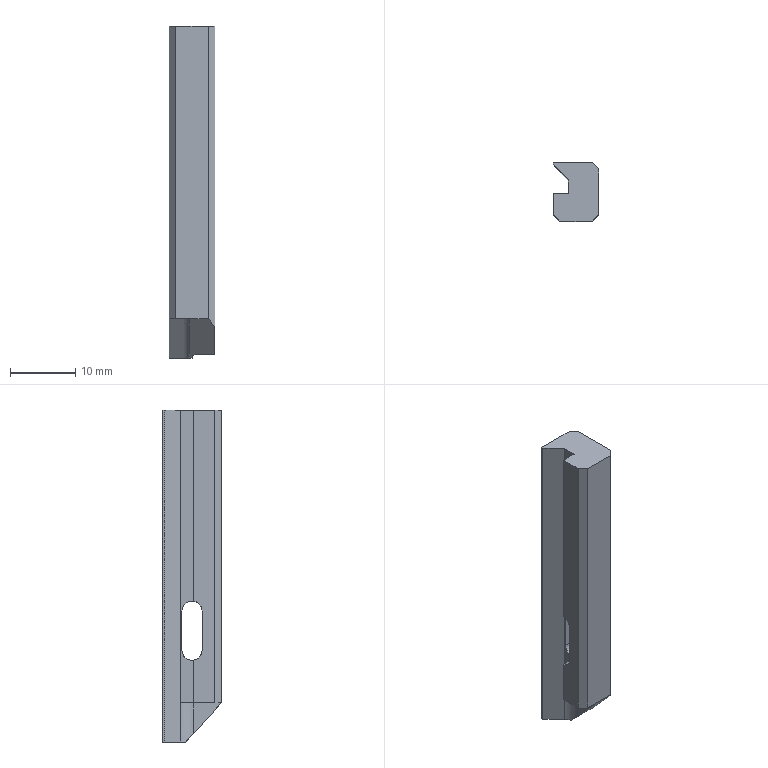Part | STEP file | 03-14 trimming upper-right blade | 1 solid | 30 faces | box 7 x 9 x 51 mm | volume 2452 mm3 | plane 22 | cylinder 8 | commonest cylinder face diameters 0.7 x4 3.1 x2 1 x1 6 x1
STEP:
#1=CARTESIAN_POINT('',(0.2245,4.1,1.));
#2=VERTEX_POINT('',#1);
#3=CARTESIAN_POINT('',(-0.4755,4.1,1.));
#4=VERTEX_POINT('',#3);
#5=CARTESIAN_POINT('',(-0.1255,4.1,1.));
#6=DIRECTION('',(0.,0.,-1.));
#7=DIRECTION('',(-1.,0.,0.));
#8=AXIS2_PLACEMENT_3D('',#5,#6,#7);
#9=CIRCLE('',#8,0.35);
#10=EDGE_CURVE('',#2,#4,#9,.T.);
#11=ORIENTED_EDGE('',*,*,#10,.F.);
#12=CARTESIAN_POINT('',(0.2245,4.1,0.));
#13=VERTEX_POINT('',#12);
#14=CARTESIAN_POINT('',(0.2245,4.1,1.));
#15=DIRECTION('',(0.,0.,-1.));
#16=VECTOR('',#15,1000.);
#17=LINE('',#14,#16);
#18=EDGE_CURVE('',#2,#13,#17,.T.);
#19=ORIENTED_EDGE('',*,*,#18,.T.);
#20=CARTESIAN_POINT('',(-0.4755,4.1,0.));
#21=VERTEX_POINT('',#20);
#22=CARTESIAN_POINT('',(-0.1255,4.1,0.));
#23=DIRECTION('',(0.,0.,-1.));
#24=DIRECTION('',(-1.,0.,0.));
#25=AXIS2_PLACEMENT_3D('',#22,#23,#24);
#26=CIRCLE('',#25,0.35);
#27=EDGE_CURVE('',#13,#21,#26,.T.);
#28=ORIENTED_EDGE('',*,*,#27,.T.);
#29=CARTESIAN_POINT('',(-0.4755,4.1,1.));
#30=DIRECTION('',(0.,0.,-1.));
#31=VECTOR('',#30,1000.);
#32=LINE('',#29,#31);
#33=EDGE_CURVE('',#4,#21,#32,.T.);
#34=ORIENTED_EDGE('',*,*,#33,.F.);
#35=EDGE_LOOP('',(#11,#19,#28,#34));
#36=FACE_OUTER_BOUND('',#35,.T.);
#37=CARTESIAN_POINT('',(-0.1255,4.1,1.));
#38=DIRECTION('',(0.,0.,-1.));
#39=DIRECTION('',(-1.,0.,0.));
#40=AXIS2_PLACEMENT_3D('',#37,#38,#39);
#41=CYLINDRICAL_SURFACE('',#40,0.35);
#42=ADVANCED_FACE('',(#36),#41,.F.);
#43=CARTESIAN_POINT('',(1.524,4.1,1.));
#44=VERTEX_POINT('',#43);
#45=CARTESIAN_POINT('',(0.8245,4.1,1.));
#46=VERTEX_POINT('',#45);
#47=CARTESIAN_POINT('',(1.174,4.1,1.));
#48=DIRECTION('',(0.,0.,-1.));
#49=DIRECTION('',(-1.,0.,0.));
#50=AXIS2_PLACEMENT_3D('',#47,#48,#49);
#51=CIRCLE('',#50,0.35);
#52=EDGE_CURVE('',#44,#46,#51,.T.);
#53=ORIENTED_EDGE('',*,*,#52,.F.);
#54=CARTESIAN_POINT('',(1.524,4.1,0.));
#55=VERTEX_POINT('',#54);
#56=CARTESIAN_POINT('',(1.524,4.1,1.));
#57=DIRECTION('',(0.,0.,-1.));
#58=VECTOR('',#57,1000.);
#59=LINE('',#56,#58);
#60=EDGE_CURVE('',#44,#55,#59,.T.);
#61=ORIENTED_EDGE('',*,*,#60,.T.);
#62=CARTESIAN_POINT('',(0.8245,4.1,0.));
#63=VERTEX_POINT('',#62);
#64=CARTESIAN_POINT('',(1.174,4.1,0.));
#65=DIRECTION('',(0.,0.,-1.));
#66=DIRECTION('',(-1.,0.,0.));
#67=AXIS2_PLACEMENT_3D('',#64,#65,#66);
#68=CIRCLE('',#67,0.35);
#69=EDGE_CURVE('',#55,#63,#68,.T.);
#70=ORIENTED_EDGE('',*,*,#69,.T.);
#71=CARTESIAN_POINT('',(0.8245,4.1,1.));
#72=DIRECTION('',(0.,0.,-1.));
#73=VECTOR('',#72,1000.);
#74=LINE('',#71,#73);
#75=EDGE_CURVE('',#46,#63,#74,.T.);
#76=ORIENTED_EDGE('',*,*,#75,.F.);
#77=EDGE_LOOP('',(#53,#61,#70,#76));
#78=FACE_OUTER_BOUND('',#77,.T.);
#79=CARTESIAN_POINT('',(1.174,4.1,1.));
#80=DIRECTION('',(0.,0.,-1.));
#81=DIRECTION('',(-1.,0.,0.));
#82=AXIS2_PLACEMENT_3D('',#79,#80,#81);
#83=CYLINDRICAL_SURFACE('',#82,0.35);
#84=ADVANCED_FACE('',(#78),#83,.F.);
#85=CARTESIAN_POINT('',(1.311,-0.2729,51.));
#86=VERTEX_POINT('',#85);
#87=CARTESIAN_POINT('',(1.311,-0.2729,21.626));
#88=VERTEX_POINT('',#87);
#89=CARTESIAN_POINT('',(1.311,-0.2729,51.));
#90=DIRECTION('',(0.,0.,-1.));
#91=VECTOR('',#90,1000.);
#92=LINE('',#89,#91);
#93=EDGE_CURVE('',#86,#88,#92,.T.);
#94=ORIENTED_EDGE('',*,*,#93,.T.);
#95=CARTESIAN_POINT('',(-1.,-0.2729,21.626));
#96=VERTEX_POINT('',#95);
#97=CARTESIAN_POINT('',(-16.,-0.2729,21.626));
#98=DIRECTION('',(-1.,0.,0.));
#99=VECTOR('',#98,1000.);
#100=LINE('',#97,#99);
#101=EDGE_CURVE('',#88,#96,#100,.T.);
#102=ORIENTED_EDGE('',*,*,#101,.T.);
#103=CARTESIAN_POINT('',(-1.,-0.2729,51.));
#104=VERTEX_POINT('',#103);
#105=CARTESIAN_POINT('',(-1.,-0.2729,51.));
#106=DIRECTION('',(0.,0.,1.));
#107=VECTOR('',#106,1000.);
#108=LINE('',#105,#107);
#109=EDGE_CURVE('',#96,#104,#108,.T.);
#110=ORIENTED_EDGE('',*,*,#109,.T.);
#111=CARTESIAN_POINT('',(1.311,-0.2729,51.));
#112=DIRECTION('',(-1.,0.,0.));
#113=VECTOR('',#112,1000.);
#114=LINE('',#111,#113);
#115=EDGE_CURVE('',#86,#104,#114,.T.);
#116=ORIENTED_EDGE('',*,*,#115,.F.);
#117=EDGE_LOOP('',(#94,#102,#110,#116));
#118=FACE_OUTER_BOUND('',#117,.T.);
#119=CARTESIAN_POINT('',(1.311,-0.2729,51.));
#120=DIRECTION('',(0.,-1.,0.));
#121=DIRECTION('',(1.,0.,0.));
#122=AXIS2_PLACEMENT_3D('',#119,#120,#121);
#123=PLANE('',#122);
#124=ADVANCED_FACE('',(#118),#123,.F.);
#125=CARTESIAN_POINT('',(5.,4.5,51.));
#126=VERTEX_POINT('',#125);
#127=CARTESIAN_POINT('',(5.,4.5,0.5));
#128=VERTEX_POINT('',#127);
#129=CARTESIAN_POINT('',(5.,4.5,51.));
#130=DIRECTION('',(0.,0.,-1.));
#131=VECTOR('',#130,1000.);
#132=LINE('',#129,#131);
#133=EDGE_CURVE('',#126,#128,#132,.T.);
#134=ORIENTED_EDGE('',*,*,#133,.T.);
#135=CARTESIAN_POINT('',(3.,4.5,0.5));
#136=VERTEX_POINT('',#135);
#137=CARTESIAN_POINT('',(6.,4.5,0.5));
#138=DIRECTION('',(1.,0.,0.));
#139=VECTOR('',#138,1000.);
#140=LINE('',#137,#139);
#141=EDGE_CURVE('',#136,#128,#140,.T.);
#142=ORIENTED_EDGE('',*,*,#141,.F.);
#143=CARTESIAN_POINT('',(2.5,4.5,0.));
#144=VERTEX_POINT('',#143);
#145=CARTESIAN_POINT('',(3.,4.5,0.));
#146=DIRECTION('',(0.,-1.,0.));
#147=DIRECTION('',(0.,0.,-1.));
#148=AXIS2_PLACEMENT_3D('',#145,#146,#147);
#149=CIRCLE('',#148,0.5);
#150=EDGE_CURVE('',#136,#144,#149,.T.);
#151=ORIENTED_EDGE('',*,*,#150,.T.);
#152=CARTESIAN_POINT('',(-1.,4.5,0.));
#153=VERTEX_POINT('',#152);
#154=CARTESIAN_POINT('',(-6.,4.5,0.));
#155=DIRECTION('',(-1.,0.,0.));
#156=VECTOR('',#155,1000.);
#157=LINE('',#154,#156);
#158=EDGE_CURVE('',#144,#153,#157,.T.);
#159=ORIENTED_EDGE('',*,*,#158,.T.);
#160=CARTESIAN_POINT('',(-1.,4.5,51.));
#161=VERTEX_POINT('',#160);
#162=CARTESIAN_POINT('',(-1.,4.5,51.));
#163=DIRECTION('',(0.,0.,-1.));
#164=VECTOR('',#163,1000.);
#165=LINE('',#162,#164);
#166=EDGE_CURVE('',#161,#153,#165,.T.);
#167=ORIENTED_EDGE('',*,*,#166,.F.);
#168=CARTESIAN_POINT('',(-6.,4.5,51.));
#169=DIRECTION('',(-1.,0.,0.));
#170=VECTOR('',#169,1000.);
#171=LINE('',#168,#170);
#172=EDGE_CURVE('',#126,#161,#171,.T.);
#173=ORIENTED_EDGE('',*,*,#172,.F.);
#174=EDGE_LOOP('',(#134,#142,#151,#159,#167,#173));
#175=FACE_OUTER_BOUND('',#174,.T.);
#176=CARTESIAN_POINT('',(-6.,4.5,51.));
#177=DIRECTION('',(0.,-1.,0.));
#178=DIRECTION('',(0.,0.,-1.));
#179=AXIS2_PLACEMENT_3D('',#176,#177,#178);
#180=PLANE('',#179);
#181=ADVANCED_FACE('',(#175),#180,.F.);
#182=CARTESIAN_POINT('',(-0.1255,4.1,0.));
#183=DIRECTION('',(0.,0.,-1.));
#184=DIRECTION('',(-1.,0.,0.));
#185=AXIS2_PLACEMENT_3D('',#182,#183,#184);
#186=CIRCLE('',#185,0.35);
#187=EDGE_CURVE('',#21,#13,#186,.T.);
#188=ORIENTED_EDGE('',*,*,#187,.F.);
#189=ORIENTED_EDGE('',*,*,#27,.F.);
#190=EDGE_LOOP('',(#188,#189));
#191=FACE_BOUND('',#190,.T.);
#192=CARTESIAN_POINT('',(1.174,4.1,0.));
#193=DIRECTION('',(0.,0.,-1.));
#194=DIRECTION('',(-1.,0.,0.));
#195=AXIS2_PLACEMENT_3D('',#192,#193,#194);
#196=CIRCLE('',#195,0.35);
#197=EDGE_CURVE('',#63,#55,#196,.T.);
#198=ORIENTED_EDGE('',*,*,#197,.F.);
#199=ORIENTED_EDGE('',*,*,#69,.F.);
#200=EDGE_LOOP('',(#198,#199));
#201=FACE_BOUND('',#200,.T.);
#202=ORIENTED_EDGE('',*,*,#158,.F.);
#203=CARTESIAN_POINT('',(2.5,0.9407,0.));
#204=VERTEX_POINT('',#203);
#205=CARTESIAN_POINT('',(2.5,-0.5,0.));
#206=DIRECTION('',(0.,1.,0.));
#207=VECTOR('',#206,1000.);
#208=LINE('',#205,#207);
#209=EDGE_CURVE('',#204,#144,#208,.T.);
#210=ORIENTED_EDGE('',*,*,#209,.F.);
#211=CARTESIAN_POINT('',(1.899,0.9407,0.));
#212=VERTEX_POINT('',#211);
#213=CARTESIAN_POINT('',(6.663,0.9407,0.));
#214=DIRECTION('',(1.,0.,0.));
#215=VECTOR('',#214,1000.);
#216=LINE('',#213,#215);
#217=EDGE_CURVE('',#212,#204,#216,.T.);
#218=ORIENTED_EDGE('',*,*,#217,.F.);
#219=CARTESIAN_POINT('',(1.311,1.813,0.));
#220=VERTEX_POINT('',#219);
#221=CARTESIAN_POINT('',(-0.8447,-0.2729,0.));
#222=DIRECTION('',(0.,0.,1.));
#223=DIRECTION('',(1.,0.,0.));
#224=AXIS2_PLACEMENT_3D('',#221,#222,#223);
#225=CIRCLE('',#224,3.);
#226=EDGE_CURVE('',#212,#220,#225,.T.);
#227=ORIENTED_EDGE('',*,*,#226,.T.);
#228=CARTESIAN_POINT('',(-1.,4.202,0.));
#229=VERTEX_POINT('',#228);
#230=CARTESIAN_POINT('',(6.733,-3.791,0.));
#231=DIRECTION('',(-0.6953,0.7187,0.));
#232=VECTOR('',#231,1000.);
#233=LINE('',#230,#232);
#234=EDGE_CURVE('',#220,#229,#233,.T.);
#235=ORIENTED_EDGE('',*,*,#234,.T.);
#236=CARTESIAN_POINT('',(-1.,-4.5,0.));
#237=DIRECTION('',(0.,-1.,0.));
#238=VECTOR('',#237,1000.);
#239=LINE('',#236,#238);
#240=EDGE_CURVE('',#153,#229,#239,.T.);
#241=ORIENTED_EDGE('',*,*,#240,.F.);
#242=EDGE_LOOP('',(#202,#210,#218,#227,#235,#241));
#243=FACE_OUTER_BOUND('',#242,.T.);
#244=CARTESIAN_POINT('',(6.,-4.5,0.));
#245=DIRECTION('',(0.,0.,1.));
#246=DIRECTION('',(1.,0.,0.));
#247=AXIS2_PLACEMENT_3D('',#244,#245,#246);
#248=PLANE('',#247);
#249=ADVANCED_FACE('',(#191,#201,#243),#248,.F.);
#250=ORIENTED_EDGE('',*,*,#234,.F.);
#251=CARTESIAN_POINT('',(1.311,1.813,6.));
#252=VERTEX_POINT('',#251);
#253=CARTESIAN_POINT('',(1.311,1.813,6.));
#254=DIRECTION('',(0.,0.,1.));
#255=VECTOR('',#254,1000.);
#256=LINE('',#253,#255);
#257=EDGE_CURVE('',#220,#252,#256,.T.);
#258=ORIENTED_EDGE('',*,*,#257,.T.);
#259=CARTESIAN_POINT('',(1.311,1.813,51.));
#260=VERTEX_POINT('',#259);
#261=CARTESIAN_POINT('',(1.311,1.813,51.));
#262=DIRECTION('',(0.,0.,-1.));
#263=VECTOR('',#262,1000.);
#264=LINE('',#261,#263);
#265=EDGE_CURVE('',#260,#252,#264,.T.);
#266=ORIENTED_EDGE('',*,*,#265,.F.);
#267=CARTESIAN_POINT('',(-1.,4.202,51.));
#268=VERTEX_POINT('',#267);
#269=CARTESIAN_POINT('',(-1.,4.202,51.));
#270=DIRECTION('',(0.6953,-0.7187,0.));
#271=VECTOR('',#270,1000.);
#272=LINE('',#269,#271);
#273=EDGE_CURVE('',#268,#260,#272,.T.);
#274=ORIENTED_EDGE('',*,*,#273,.F.);
#275=CARTESIAN_POINT('',(-1.,4.202,6.));
#276=DIRECTION('',(0.,0.,1.));
#277=VECTOR('',#276,1000.);
#278=LINE('',#275,#277);
#279=EDGE_CURVE('',#229,#268,#278,.T.);
#280=ORIENTED_EDGE('',*,*,#279,.F.);
#281=EDGE_LOOP('',(#250,#258,#266,#274,#280));
#282=FACE_OUTER_BOUND('',#281,.T.);
#283=CARTESIAN_POINT('',(-2.682,5.941,6.));
#284=DIRECTION('',(0.7187,0.6953,0.));
#285=DIRECTION('',(-0.6953,0.7187,0.));
#286=AXIS2_PLACEMENT_3D('',#283,#284,#285);
#287=PLANE('',#286);
#288=ADVANCED_FACE('',(#282),#287,.F.);
#289=CARTESIAN_POINT('',(6.,0.4873,0.5));
#290=VERTEX_POINT('',#289);
#291=CARTESIAN_POINT('',(3.,0.4873,0.5));
#292=VERTEX_POINT('',#291);
#293=CARTESIAN_POINT('',(-6.,0.4873,0.5));
#294=DIRECTION('',(-1.,0.,0.));
#295=VECTOR('',#294,1000.);
#296=LINE('',#293,#295);
#297=EDGE_CURVE('',#290,#292,#296,.T.);
#298=ORIENTED_EDGE('',*,*,#297,.F.);
#299=CARTESIAN_POINT('',(6.,-3.5,4.897));
#300=VERTEX_POINT('',#299);
#301=CARTESIAN_POINT('',(6.,0.9407,0.));
#302=DIRECTION('',(0.,0.6717,-0.7408));
#303=VECTOR('',#302,1000.);
#304=LINE('',#301,#303);
#305=EDGE_CURVE('',#300,#290,#304,.T.);
#306=ORIENTED_EDGE('',*,*,#305,.F.);
#307=CARTESIAN_POINT('',(5.,-4.5,6.));
#308=VERTEX_POINT('',#307);
#309=CARTESIAN_POINT('',(5.329,-4.171,5.637));
#310=DIRECTION('',(-0.5576,-0.5576,0.6149));
#311=VECTOR('',#310,1000.);
#312=LINE('',#309,#311);
#313=EDGE_CURVE('',#300,#308,#312,.T.);
#314=ORIENTED_EDGE('',*,*,#313,.T.);
#315=CARTESIAN_POINT('',(2.155,-4.5,6.));
#316=VERTEX_POINT('',#315);
#317=CARTESIAN_POINT('',(-6.,-4.5,6.));
#318=DIRECTION('',(1.,0.,0.));
#319=VECTOR('',#318,1000.);
#320=LINE('',#317,#319);
#321=EDGE_CURVE('',#316,#308,#320,.T.);
#322=ORIENTED_EDGE('',*,*,#321,.F.);
#323=CARTESIAN_POINT('',(2.155,-0.2729,1.338));
#324=VERTEX_POINT('',#323);
#325=CARTESIAN_POINT('',(2.155,0.9407,0.));
#326=DIRECTION('',(0.,0.6717,-0.7408));
#327=VECTOR('',#326,1000.);
#328=LINE('',#325,#327);
#329=EDGE_CURVE('',#316,#324,#328,.T.);
#330=ORIENTED_EDGE('',*,*,#329,.T.);
#331=CARTESIAN_POINT('',(2.155,-0.2729,1.338));
#332=CARTESIAN_POINT('',(2.155,0.1466,0.8758));
#333=CARTESIAN_POINT('',(2.069,0.5571,0.4231));
#334=CARTESIAN_POINT('',(1.899,0.9407,0.));
#335=(BOUNDED_CURVE()B_SPLINE_CURVE(3,(#331,#332,#333,#334),.UNSPECIFIED.,.F.,.F.)B_SPLINE_CURVE_WITH_KNOTS((4,4),(4.712,5.129),.UNSPECIFIED.)CURVE()GEOMETRIC_REPRESENTATION_ITEM()RATIONAL_B_SPLINE_CURVE((1.,0.9856,0.9856,1.))REPRESENTATION_ITEM(''));
#336=EDGE_CURVE('',#324,#212,#335,.T.);
#337=ORIENTED_EDGE('',*,*,#336,.T.);
#338=ORIENTED_EDGE('',*,*,#217,.T.);
#339=CARTESIAN_POINT('',(2.5,0.9407,0.));
#340=CARTESIAN_POINT('',(2.5,0.6751,0.2929));
#341=CARTESIAN_POINT('',(2.707,0.4873,0.5));
#342=CARTESIAN_POINT('',(3.,0.4873,0.5));
#343=(BOUNDED_CURVE()B_SPLINE_CURVE(3,(#339,#340,#341,#342),.UNSPECIFIED.,.F.,.F.)B_SPLINE_CURVE_WITH_KNOTS((4,4),(4.712,6.283),.UNSPECIFIED.)CURVE()GEOMETRIC_REPRESENTATION_ITEM()RATIONAL_B_SPLINE_CURVE((1.,0.8047,0.8047,1.))REPRESENTATION_ITEM(''));
#344=EDGE_CURVE('',#204,#292,#343,.T.);
#345=ORIENTED_EDGE('',*,*,#344,.T.);
#346=EDGE_LOOP('',(#298,#306,#314,#322,#330,#337,#338,#345));
#347=FACE_OUTER_BOUND('',#346,.T.);
#348=CARTESIAN_POINT('',(-6.,0.9407,0.));
#349=DIRECTION('',(0.,-0.7408,-0.6717));
#350=DIRECTION('',(0.,0.6717,-0.7408));
#351=AXIS2_PLACEMENT_3D('',#348,#349,#350);
#352=PLANE('',#351);
#353=ADVANCED_FACE('',(#347),#352,.T.);
#354=CARTESIAN_POINT('',(6.,-1.55,20.1));
#355=VERTEX_POINT('',#354);
#356=CARTESIAN_POINT('',(6.,-1.55,14.1));
#357=VERTEX_POINT('',#356);
#358=CARTESIAN_POINT('',(6.,-1.55,20.1));
#359=DIRECTION('',(0.,0.,-1.));
#360=VECTOR('',#359,1000.);
#361=LINE('',#358,#360);
#362=EDGE_CURVE('',#355,#357,#361,.T.);
#363=ORIENTED_EDGE('',*,*,#362,.F.);
#364=CARTESIAN_POINT('',(6.,1.55,20.1));
#365=VERTEX_POINT('',#364);
#366=CARTESIAN_POINT('',(6.,0.,20.1));
#367=DIRECTION('',(1.,0.,0.));
#368=DIRECTION('',(0.,1.,0.));
#369=AXIS2_PLACEMENT_3D('',#366,#367,#368);
#370=CIRCLE('',#369,1.55);
#371=EDGE_CURVE('',#365,#355,#370,.T.);
#372=ORIENTED_EDGE('',*,*,#371,.F.);
#373=CARTESIAN_POINT('',(6.,1.55,14.1));
#374=VERTEX_POINT('',#373);
#375=CARTESIAN_POINT('',(6.,1.55,20.1));
#376=DIRECTION('',(0.,0.,1.));
#377=VECTOR('',#376,1000.);
#378=LINE('',#375,#377);
#379=EDGE_CURVE('',#374,#365,#378,.T.);
#380=ORIENTED_EDGE('',*,*,#379,.F.);
#381=CARTESIAN_POINT('',(6.,0.,14.1));
#382=DIRECTION('',(1.,0.,0.));
#383=DIRECTION('',(0.,1.,0.));
#384=AXIS2_PLACEMENT_3D('',#381,#382,#383);
#385=CIRCLE('',#384,1.55);
#386=EDGE_CURVE('',#357,#374,#385,.T.);
#387=ORIENTED_EDGE('',*,*,#386,.F.);
#388=EDGE_LOOP('',(#363,#372,#380,#387));
#389=FACE_BOUND('',#388,.T.);
#390=ORIENTED_EDGE('',*,*,#305,.T.);
#391=CARTESIAN_POINT('',(6.,3.5,0.5));
#392=VERTEX_POINT('',#391);
#393=CARTESIAN_POINT('',(6.,-0.5,0.5));
#394=DIRECTION('',(0.,1.,0.));
#395=VECTOR('',#394,1000.);
#396=LINE('',#393,#395);
#397=EDGE_CURVE('',#290,#392,#396,.T.);
#398=ORIENTED_EDGE('',*,*,#397,.T.);
#399=CARTESIAN_POINT('',(6.,3.5,51.));
#400=VERTEX_POINT('',#399);
#401=CARTESIAN_POINT('',(6.,3.5,51.));
#402=DIRECTION('',(0.,0.,1.));
#403=VECTOR('',#402,1000.);
#404=LINE('',#401,#403);
#405=EDGE_CURVE('',#392,#400,#404,.T.);
#406=ORIENTED_EDGE('',*,*,#405,.T.);
#407=CARTESIAN_POINT('',(6.,-3.5,51.));
#408=VERTEX_POINT('',#407);
#409=CARTESIAN_POINT('',(6.,4.5,51.));
#410=DIRECTION('',(0.,1.,0.));
#411=VECTOR('',#410,1000.);
#412=LINE('',#409,#411);
#413=EDGE_CURVE('',#408,#400,#412,.T.);
#414=ORIENTED_EDGE('',*,*,#413,.F.);
#415=CARTESIAN_POINT('',(6.,-3.5,51.));
#416=DIRECTION('',(0.,0.,-1.));
#417=VECTOR('',#416,1000.);
#418=LINE('',#415,#417);
#419=EDGE_CURVE('',#408,#300,#418,.T.);
#420=ORIENTED_EDGE('',*,*,#419,.T.);
#421=EDGE_LOOP('',(#390,#398,#406,#414,#420));
#422=FACE_OUTER_BOUND('',#421,.T.);
#423=CARTESIAN_POINT('',(6.,4.5,51.));
#424=DIRECTION('',(-1.,0.,0.));
#425=DIRECTION('',(0.,-1.,0.));
#426=AXIS2_PLACEMENT_3D('',#423,#424,#425);
#427=PLANE('',#426);
#428=ADVANCED_FACE('',(#389,#422),#427,.F.);
#429=CARTESIAN_POINT('',(0.,-4.5,51.));
#430=VERTEX_POINT('',#429);
#431=CARTESIAN_POINT('',(5.,-4.5,51.));
#432=VERTEX_POINT('',#431);
#433=CARTESIAN_POINT('',(-6.,-4.5,51.));
#434=DIRECTION('',(1.,0.,0.));
#435=VECTOR('',#434,1000.);
#436=LINE('',#433,#435);
#437=EDGE_CURVE('',#430,#432,#436,.T.);
#438=ORIENTED_EDGE('',*,*,#437,.F.);
#439=CARTESIAN_POINT('',(0.,-4.5,6.));
#440=VERTEX_POINT('',#439);
#441=CARTESIAN_POINT('',(0.,-4.5,51.));
#442=DIRECTION('',(0.,0.,-1.));
#443=VECTOR('',#442,1000.);
#444=LINE('',#441,#443);
#445=EDGE_CURVE('',#430,#440,#444,.T.);
#446=ORIENTED_EDGE('',*,*,#445,.T.);
#447=CARTESIAN_POINT('',(-6.,-4.5,6.));
#448=DIRECTION('',(1.,0.,0.));
#449=VECTOR('',#448,1000.);
#450=LINE('',#447,#449);
#451=EDGE_CURVE('',#440,#316,#450,.T.);
#452=ORIENTED_EDGE('',*,*,#451,.T.);
#453=ORIENTED_EDGE('',*,*,#321,.T.);
#454=CARTESIAN_POINT('',(5.,-4.5,51.));
#455=DIRECTION('',(0.,0.,1.));
#456=VECTOR('',#455,1000.);
#457=LINE('',#454,#456);
#458=EDGE_CURVE('',#308,#432,#457,.T.);
#459=ORIENTED_EDGE('',*,*,#458,.T.);
#460=EDGE_LOOP('',(#438,#446,#452,#453,#459));
#461=FACE_OUTER_BOUND('',#460,.T.);
#462=CARTESIAN_POINT('',(-6.,-4.5,51.));
#463=DIRECTION('',(0.,1.,0.));
#464=DIRECTION('',(0.,0.,1.));
#465=AXIS2_PLACEMENT_3D('',#462,#463,#464);
#466=PLANE('',#465);
#467=ADVANCED_FACE('',(#461),#466,.F.);
#468=CARTESIAN_POINT('',(-1.,-3.5,51.));
#469=VERTEX_POINT('',#468);
#470=CARTESIAN_POINT('',(-1.,4.5,51.));
#471=DIRECTION('',(0.,1.,0.));
#472=VECTOR('',#471,1000.);
#473=LINE('',#470,#472);
#474=EDGE_CURVE('',#469,#104,#473,.T.);
#475=ORIENTED_EDGE('',*,*,#474,.F.);
#476=CARTESIAN_POINT('',(3.,-7.5,51.));
#477=DIRECTION('',(0.7071,-0.7071,0.));
#478=VECTOR('',#477,1000.);
#479=LINE('',#476,#478);
#480=EDGE_CURVE('',#469,#430,#479,.T.);
#481=ORIENTED_EDGE('',*,*,#480,.T.);
#482=ORIENTED_EDGE('',*,*,#437,.T.);
#483=CARTESIAN_POINT('',(5.5,-4.,51.));
#484=DIRECTION('',(0.7071,0.7071,0.));
#485=VECTOR('',#484,1000.);
#486=LINE('',#483,#485);
#487=EDGE_CURVE('',#432,#408,#486,.T.);
#488=ORIENTED_EDGE('',*,*,#487,.T.);
#489=ORIENTED_EDGE('',*,*,#413,.T.);
#490=CARTESIAN_POINT('',(10.,-0.5,51.));
#491=DIRECTION('',(-0.7071,0.7071,0.));
#492=VECTOR('',#491,1000.);
#493=LINE('',#490,#492);
#494=EDGE_CURVE('',#400,#126,#493,.T.);
#495=ORIENTED_EDGE('',*,*,#494,.T.);
#496=ORIENTED_EDGE('',*,*,#172,.T.);
#497=CARTESIAN_POINT('',(-1.,4.5,51.));
#498=DIRECTION('',(0.,-1.,0.));
#499=VECTOR('',#498,1000.);
#500=LINE('',#497,#499);
#501=EDGE_CURVE('',#161,#268,#500,.T.);
#502=ORIENTED_EDGE('',*,*,#501,.T.);
#503=ORIENTED_EDGE('',*,*,#273,.T.);
#504=CARTESIAN_POINT('',(1.311,1.813,51.));
#505=DIRECTION('',(0.,-1.,0.));
#506=VECTOR('',#505,1000.);
#507=LINE('',#504,#506);
#508=EDGE_CURVE('',#260,#86,#507,.T.);
#509=ORIENTED_EDGE('',*,*,#508,.T.);
#510=ORIENTED_EDGE('',*,*,#115,.T.);
#511=EDGE_LOOP('',(#475,#481,#482,#488,#489,#495,#496,#502,#503,#509,#510));
#512=FACE_OUTER_BOUND('',#511,.T.);
#513=CARTESIAN_POINT('',(6.,-4.5,51.));
#514=DIRECTION('',(0.,0.,1.));
#515=DIRECTION('',(1.,0.,0.));
#516=AXIS2_PLACEMENT_3D('',#513,#514,#515);
#517=PLANE('',#516);
#518=ADVANCED_FACE('',(#512),#517,.T.);
#519=ORIENTED_EDGE('',*,*,#451,.F.);
#520=CARTESIAN_POINT('',(-1.,-3.5,6.));
#521=VERTEX_POINT('',#520);
#522=CARTESIAN_POINT('',(0.,-4.5,6.));
#523=DIRECTION('',(-0.7071,0.7071,0.));
#524=VECTOR('',#523,1000.);
#525=LINE('',#522,#524);
#526=EDGE_CURVE('',#440,#521,#525,.T.);
#527=ORIENTED_EDGE('',*,*,#526,.T.);
#528=CARTESIAN_POINT('',(-1.,-0.2729,6.));
#529=VERTEX_POINT('',#528);
#530=CARTESIAN_POINT('',(-1.,5.941,6.));
#531=DIRECTION('',(0.,1.,0.));
#532=VECTOR('',#531,1000.);
#533=LINE('',#530,#532);
#534=EDGE_CURVE('',#521,#529,#533,.T.);
#535=ORIENTED_EDGE('',*,*,#534,.T.);
#536=CARTESIAN_POINT('',(1.311,-0.2729,6.));
#537=VERTEX_POINT('',#536);
#538=CARTESIAN_POINT('',(1.311,-0.2729,6.));
#539=DIRECTION('',(-1.,0.,0.));
#540=VECTOR('',#539,1000.);
#541=LINE('',#538,#540);
#542=EDGE_CURVE('',#537,#529,#541,.T.);
#543=ORIENTED_EDGE('',*,*,#542,.F.);
#544=CARTESIAN_POINT('',(1.311,1.813,6.));
#545=DIRECTION('',(0.,-1.,0.));
#546=VECTOR('',#545,1000.);
#547=LINE('',#544,#546);
#548=EDGE_CURVE('',#252,#537,#547,.T.);
#549=ORIENTED_EDGE('',*,*,#548,.F.);
#550=CARTESIAN_POINT('',(2.155,-0.2729,6.));
#551=VERTEX_POINT('',#550);
#552=CARTESIAN_POINT('',(-0.8447,-0.2729,6.));
#553=DIRECTION('',(0.,0.,-1.));
#554=DIRECTION('',(1.,0.,0.));
#555=AXIS2_PLACEMENT_3D('',#552,#553,#554);
#556=CIRCLE('',#555,3.);
#557=EDGE_CURVE('',#252,#551,#556,.T.);
#558=ORIENTED_EDGE('',*,*,#557,.T.);
#559=CARTESIAN_POINT('',(2.155,0.9407,6.));
#560=DIRECTION('',(0.,-1.,0.));
#561=VECTOR('',#560,1000.);
#562=LINE('',#559,#561);
#563=EDGE_CURVE('',#551,#316,#562,.T.);
#564=ORIENTED_EDGE('',*,*,#563,.T.);
#565=EDGE_LOOP('',(#519,#527,#535,#543,#549,#558,#564));
#566=FACE_OUTER_BOUND('',#565,.T.);
#567=CARTESIAN_POINT('',(-7.387,5.941,6.));
#568=DIRECTION('',(0.,0.,1.));
#569=DIRECTION('',(1.,0.,0.));
#570=AXIS2_PLACEMENT_3D('',#567,#568,#569);
#571=PLANE('',#570);
#572=ADVANCED_FACE('',(#566),#571,.F.);
#573=ORIENTED_EDGE('',*,*,#563,.F.);
#574=CARTESIAN_POINT('',(2.155,-0.2729,-6.));
#575=DIRECTION('',(0.,0.,-1.));
#576=VECTOR('',#575,1000.);
#577=LINE('',#574,#576);
#578=EDGE_CURVE('',#551,#324,#577,.T.);
#579=ORIENTED_EDGE('',*,*,#578,.T.);
#580=ORIENTED_EDGE('',*,*,#329,.F.);
#581=EDGE_LOOP('',(#573,#579,#580));
#582=FACE_OUTER_BOUND('',#581,.T.);
#583=CARTESIAN_POINT('',(2.155,0.9407,-6.));
#584=DIRECTION('',(-1.,0.,0.));
#585=DIRECTION('',(0.,0.,1.));
#586=AXIS2_PLACEMENT_3D('',#583,#584,#585);
#587=PLANE('',#586);
#588=ADVANCED_FACE('',(#582),#587,.T.);
#589=ORIENTED_EDGE('',*,*,#166,.T.);
#590=ORIENTED_EDGE('',*,*,#240,.T.);
#591=ORIENTED_EDGE('',*,*,#279,.T.);
#592=ORIENTED_EDGE('',*,*,#501,.F.);
#593=EDGE_LOOP('',(#589,#590,#591,#592));
#594=FACE_OUTER_BOUND('',#593,.T.);
#595=CARTESIAN_POINT('',(-1.,5.514,-6.));
#596=DIRECTION('',(-1.,0.,0.));
#597=DIRECTION('',(0.,-1.,0.));
#598=AXIS2_PLACEMENT_3D('',#595,#596,#597);
#599=PLANE('',#598);
#600=ADVANCED_FACE('',(#594),#599,.T.);
#601=ORIENTED_EDGE('',*,*,#557,.F.);
#602=ORIENTED_EDGE('',*,*,#257,.F.);
#603=ORIENTED_EDGE('',*,*,#226,.F.);
#604=ORIENTED_EDGE('',*,*,#336,.F.);
#605=ORIENTED_EDGE('',*,*,#578,.F.);
#606=EDGE_LOOP('',(#601,#602,#603,#604,#605));
#607=FACE_OUTER_BOUND('',#606,.T.);
#608=CARTESIAN_POINT('',(-0.8447,-0.2729,-6.));
#609=DIRECTION('',(0.,0.,-1.));
#610=DIRECTION('',(-1.,0.,0.));
#611=AXIS2_PLACEMENT_3D('',#608,#609,#610);
#612=CYLINDRICAL_SURFACE('',#611,3.);
#613=ADVANCED_FACE('',(#607),#612,.F.);
#614=ORIENTED_EDGE('',*,*,#487,.F.);
#615=ORIENTED_EDGE('',*,*,#458,.F.);
#616=ORIENTED_EDGE('',*,*,#313,.F.);
#617=ORIENTED_EDGE('',*,*,#419,.F.);
#618=EDGE_LOOP('',(#614,#615,#616,#617));
#619=FACE_OUTER_BOUND('',#618,.T.);
#620=CARTESIAN_POINT('',(6.,-3.5,51.));
#621=DIRECTION('',(-0.7071,0.7071,0.));
#622=DIRECTION('',(-0.7071,-0.7071,0.));
#623=AXIS2_PLACEMENT_3D('',#620,#621,#622);
#624=PLANE('',#623);
#625=ADVANCED_FACE('',(#619),#624,.F.);
#626=CARTESIAN_POINT('',(5.,4.5,0.5));
#627=DIRECTION('',(0.7071,-0.7071,0.));
#628=VECTOR('',#627,1000.);
#629=LINE('',#626,#628);
#630=EDGE_CURVE('',#128,#392,#629,.T.);
#631=ORIENTED_EDGE('',*,*,#630,.F.);
#632=ORIENTED_EDGE('',*,*,#133,.F.);
#633=ORIENTED_EDGE('',*,*,#494,.F.);
#634=ORIENTED_EDGE('',*,*,#405,.F.);
#635=EDGE_LOOP('',(#631,#632,#633,#634));
#636=FACE_OUTER_BOUND('',#635,.T.);
#637=CARTESIAN_POINT('',(5.,4.5,51.));
#638=DIRECTION('',(-0.7071,-0.7071,0.));
#639=DIRECTION('',(0.7071,-0.7071,0.));
#640=AXIS2_PLACEMENT_3D('',#637,#638,#639);
#641=PLANE('',#640);
#642=ADVANCED_FACE('',(#636),#641,.F.);
#643=CARTESIAN_POINT('',(-1.,-0.2729,12.574));
#644=VERTEX_POINT('',#643);
#645=CARTESIAN_POINT('',(-1.,-0.2729,51.));
#646=DIRECTION('',(0.,0.,1.));
#647=VECTOR('',#646,1000.);
#648=LINE('',#645,#647);
#649=EDGE_CURVE('',#529,#644,#648,.T.);
#650=ORIENTED_EDGE('',*,*,#649,.T.);
#651=CARTESIAN_POINT('',(1.311,-0.2729,12.574));
#652=VERTEX_POINT('',#651);
#653=CARTESIAN_POINT('',(-16.,-0.2729,12.574));
#654=DIRECTION('',(1.,0.,0.));
#655=VECTOR('',#654,1000.);
#656=LINE('',#653,#655);
#657=EDGE_CURVE('',#644,#652,#656,.T.);
#658=ORIENTED_EDGE('',*,*,#657,.T.);
#659=CARTESIAN_POINT('',(1.311,-0.2729,51.));
#660=DIRECTION('',(0.,0.,-1.));
#661=VECTOR('',#660,1000.);
#662=LINE('',#659,#661);
#663=EDGE_CURVE('',#652,#537,#662,.T.);
#664=ORIENTED_EDGE('',*,*,#663,.T.);
#665=ORIENTED_EDGE('',*,*,#542,.T.);
#666=EDGE_LOOP('',(#650,#658,#664,#665));
#667=FACE_OUTER_BOUND('',#666,.T.);
#668=CARTESIAN_POINT('',(1.311,-0.2729,51.));
#669=DIRECTION('',(0.,-1.,0.));
#670=DIRECTION('',(1.,0.,0.));
#671=AXIS2_PLACEMENT_3D('',#668,#669,#670);
#672=PLANE('',#671);
#673=ADVANCED_FACE('',(#667),#672,.F.);
#674=CARTESIAN_POINT('',(1.311,1.55,14.1));
#675=VERTEX_POINT('',#674);
#676=CARTESIAN_POINT('',(1.311,1.55,20.1));
#677=VERTEX_POINT('',#676);
#678=CARTESIAN_POINT('',(1.311,1.55,51.));
#679=DIRECTION('',(0.,0.,1.));
#680=VECTOR('',#679,1000.);
#681=LINE('',#678,#680);
#682=EDGE_CURVE('',#675,#677,#681,.T.);
#683=ORIENTED_EDGE('',*,*,#682,.T.);
#684=CARTESIAN_POINT('',(1.311,0.,20.1));
#685=DIRECTION('',(1.,0.,0.));
#686=DIRECTION('',(0.,0.,-1.));
#687=AXIS2_PLACEMENT_3D('',#684,#685,#686);
#688=CIRCLE('',#687,1.55);
#689=EDGE_CURVE('',#677,#88,#688,.T.);
#690=ORIENTED_EDGE('',*,*,#689,.T.);
#691=ORIENTED_EDGE('',*,*,#93,.F.);
#692=ORIENTED_EDGE('',*,*,#508,.F.);
#693=ORIENTED_EDGE('',*,*,#265,.T.);
#694=ORIENTED_EDGE('',*,*,#548,.T.);
#695=ORIENTED_EDGE('',*,*,#663,.F.);
#696=CARTESIAN_POINT('',(1.311,0.,14.1));
#697=DIRECTION('',(1.,0.,0.));
#698=DIRECTION('',(0.,0.,-1.));
#699=AXIS2_PLACEMENT_3D('',#696,#697,#698);
#700=CIRCLE('',#699,1.55);
#701=EDGE_CURVE('',#652,#675,#700,.T.);
#702=ORIENTED_EDGE('',*,*,#701,.T.);
#703=EDGE_LOOP('',(#683,#690,#691,#692,#693,#694,#695,#702));
#704=FACE_OUTER_BOUND('',#703,.T.);
#705=CARTESIAN_POINT('',(1.311,1.813,51.));
#706=DIRECTION('',(1.,0.,0.));
#707=DIRECTION('',(0.,0.,-1.));
#708=AXIS2_PLACEMENT_3D('',#705,#706,#707);
#709=PLANE('',#708);
#710=ADVANCED_FACE('',(#704),#709,.F.);
#711=ORIENTED_EDGE('',*,*,#109,.F.);
#712=CARTESIAN_POINT('',(-1.,-1.55,20.1));
#713=VERTEX_POINT('',#712);
#714=CARTESIAN_POINT('',(-1.,0.,20.1));
#715=DIRECTION('',(1.,0.,0.));
#716=DIRECTION('',(0.,0.,-1.));
#717=AXIS2_PLACEMENT_3D('',#714,#715,#716);
#718=CIRCLE('',#717,1.55);
#719=EDGE_CURVE('',#96,#713,#718,.T.);
#720=ORIENTED_EDGE('',*,*,#719,.T.);
#721=CARTESIAN_POINT('',(-1.,-1.55,14.1));
#722=VERTEX_POINT('',#721);
#723=CARTESIAN_POINT('',(-1.,-1.55,0.));
#724=DIRECTION('',(0.,0.,-1.));
#725=VECTOR('',#724,1000.);
#726=LINE('',#723,#725);
#727=EDGE_CURVE('',#713,#722,#726,.T.);
#728=ORIENTED_EDGE('',*,*,#727,.T.);
#729=CARTESIAN_POINT('',(-1.,0.,14.1));
#730=DIRECTION('',(1.,0.,0.));
#731=DIRECTION('',(0.,0.,-1.));
#732=AXIS2_PLACEMENT_3D('',#729,#730,#731);
#733=CIRCLE('',#732,1.55);
#734=EDGE_CURVE('',#722,#644,#733,.T.);
#735=ORIENTED_EDGE('',*,*,#734,.T.);
#736=ORIENTED_EDGE('',*,*,#649,.F.);
#737=ORIENTED_EDGE('',*,*,#534,.F.);
#738=CARTESIAN_POINT('',(-1.,-3.5,0.));
#739=DIRECTION('',(0.,0.,1.));
#740=VECTOR('',#739,1000.);
#741=LINE('',#738,#740);
#742=EDGE_CURVE('',#521,#469,#741,.T.);
#743=ORIENTED_EDGE('',*,*,#742,.T.);
#744=ORIENTED_EDGE('',*,*,#474,.T.);
#745=EDGE_LOOP('',(#711,#720,#728,#735,#736,#737,#743,#744));
#746=FACE_OUTER_BOUND('',#745,.T.);
#747=CARTESIAN_POINT('',(-1.,4.5,0.));
#748=DIRECTION('',(1.,0.,0.));
#749=DIRECTION('',(0.,0.,-1.));
#750=AXIS2_PLACEMENT_3D('',#747,#748,#749);
#751=PLANE('',#750);
#752=ADVANCED_FACE('',(#746),#751,.F.);
#753=ORIENTED_EDGE('',*,*,#480,.F.);
#754=ORIENTED_EDGE('',*,*,#742,.F.);
#755=ORIENTED_EDGE('',*,*,#526,.F.);
#756=ORIENTED_EDGE('',*,*,#445,.F.);
#757=EDGE_LOOP('',(#753,#754,#755,#756));
#758=FACE_OUTER_BOUND('',#757,.T.);
#759=CARTESIAN_POINT('',(0.,-4.5,51.));
#760=DIRECTION('',(0.7071,0.7071,0.));
#761=DIRECTION('',(-0.7071,0.7071,0.));
#762=AXIS2_PLACEMENT_3D('',#759,#760,#761);
#763=PLANE('',#762);
#764=ADVANCED_FACE('',(#758),#763,.F.);
#765=ORIENTED_EDGE('',*,*,#297,.T.);
#766=CARTESIAN_POINT('',(3.,4.5,0.5));
#767=DIRECTION('',(0.,1.,0.));
#768=VECTOR('',#767,1000.);
#769=LINE('',#766,#768);
#770=EDGE_CURVE('',#292,#136,#769,.T.);
#771=ORIENTED_EDGE('',*,*,#770,.T.);
#772=ORIENTED_EDGE('',*,*,#141,.T.);
#773=ORIENTED_EDGE('',*,*,#630,.T.);
#774=ORIENTED_EDGE('',*,*,#397,.F.);
#775=EDGE_LOOP('',(#765,#771,#772,#773,#774));
#776=FACE_OUTER_BOUND('',#775,.T.);
#777=CARTESIAN_POINT('',(6.,-0.5,0.5));
#778=DIRECTION('',(0.,0.,1.));
#779=DIRECTION('',(1.,0.,0.));
#780=AXIS2_PLACEMENT_3D('',#777,#778,#779);
#781=PLANE('',#780);
#782=ADVANCED_FACE('',(#776),#781,.F.);
#783=ORIENTED_EDGE('',*,*,#344,.F.);
#784=ORIENTED_EDGE('',*,*,#209,.T.);
#785=ORIENTED_EDGE('',*,*,#150,.F.);
#786=ORIENTED_EDGE('',*,*,#770,.F.);
#787=EDGE_LOOP('',(#783,#784,#785,#786));
#788=FACE_OUTER_BOUND('',#787,.T.);
#789=CARTESIAN_POINT('',(3.,-0.5,0.));
#790=DIRECTION('',(0.,-1.,0.));
#791=DIRECTION('',(0.,0.,-1.));
#792=AXIS2_PLACEMENT_3D('',#789,#790,#791);
#793=CYLINDRICAL_SURFACE('',#792,0.5);
#794=ADVANCED_FACE('',(#788),#793,.F.);
#795=CARTESIAN_POINT('',(-16.,1.55,14.1));
#796=DIRECTION('',(1.,0.,0.));
#797=VECTOR('',#796,1000.);
#798=LINE('',#795,#797);
#799=EDGE_CURVE('',#675,#374,#798,.T.);
#800=ORIENTED_EDGE('',*,*,#799,.T.);
#801=ORIENTED_EDGE('',*,*,#379,.T.);
#802=CARTESIAN_POINT('',(-16.,1.55,20.1));
#803=DIRECTION('',(1.,0.,0.));
#804=VECTOR('',#803,1000.);
#805=LINE('',#802,#804);
#806=EDGE_CURVE('',#677,#365,#805,.T.);
#807=ORIENTED_EDGE('',*,*,#806,.F.);
#808=ORIENTED_EDGE('',*,*,#682,.F.);
#809=EDGE_LOOP('',(#800,#801,#807,#808));
#810=FACE_OUTER_BOUND('',#809,.T.);
#811=CARTESIAN_POINT('',(-16.,1.55,20.1));
#812=DIRECTION('',(0.,1.,0.));
#813=DIRECTION('',(0.,0.,1.));
#814=AXIS2_PLACEMENT_3D('',#811,#812,#813);
#815=PLANE('',#814);
#816=ADVANCED_FACE('',(#810),#815,.F.);
#817=ORIENTED_EDGE('',*,*,#806,.T.);
#818=ORIENTED_EDGE('',*,*,#371,.T.);
#819=CARTESIAN_POINT('',(-16.,-1.55,20.1));
#820=DIRECTION('',(1.,0.,0.));
#821=VECTOR('',#820,1000.);
#822=LINE('',#819,#821);
#823=EDGE_CURVE('',#713,#355,#822,.T.);
#824=ORIENTED_EDGE('',*,*,#823,.F.);
#825=ORIENTED_EDGE('',*,*,#719,.F.);
#826=ORIENTED_EDGE('',*,*,#101,.F.);
#827=ORIENTED_EDGE('',*,*,#689,.F.);
#828=EDGE_LOOP('',(#817,#818,#824,#825,#826,#827));
#829=FACE_OUTER_BOUND('',#828,.T.);
#830=CARTESIAN_POINT('',(-16.,0.,20.1));
#831=DIRECTION('',(1.,0.,0.));
#832=DIRECTION('',(0.,1.,0.));
#833=AXIS2_PLACEMENT_3D('',#830,#831,#832);
#834=CYLINDRICAL_SURFACE('',#833,1.55);
#835=ADVANCED_FACE('',(#829),#834,.F.);
#836=ORIENTED_EDGE('',*,*,#657,.F.);
#837=ORIENTED_EDGE('',*,*,#734,.F.);
#838=CARTESIAN_POINT('',(-16.,-1.55,14.1));
#839=DIRECTION('',(1.,0.,0.));
#840=VECTOR('',#839,1000.);
#841=LINE('',#838,#840);
#842=EDGE_CURVE('',#722,#357,#841,.T.);
#843=ORIENTED_EDGE('',*,*,#842,.T.);
#844=ORIENTED_EDGE('',*,*,#386,.T.);
#845=ORIENTED_EDGE('',*,*,#799,.F.);
#846=ORIENTED_EDGE('',*,*,#701,.F.);
#847=EDGE_LOOP('',(#836,#837,#843,#844,#845,#846));
#848=FACE_OUTER_BOUND('',#847,.T.);
#849=CARTESIAN_POINT('',(-16.,0.,14.1));
#850=DIRECTION('',(1.,0.,0.));
#851=DIRECTION('',(0.,1.,0.));
#852=AXIS2_PLACEMENT_3D('',#849,#850,#851);
#853=CYLINDRICAL_SURFACE('',#852,1.55);
#854=ADVANCED_FACE('',(#848),#853,.F.);
#855=ORIENTED_EDGE('',*,*,#823,.T.);
#856=ORIENTED_EDGE('',*,*,#362,.T.);
#857=ORIENTED_EDGE('',*,*,#842,.F.);
#858=ORIENTED_EDGE('',*,*,#727,.F.);
#859=EDGE_LOOP('',(#855,#856,#857,#858));
#860=FACE_OUTER_BOUND('',#859,.T.);
#861=CARTESIAN_POINT('',(-16.,-1.55,20.1));
#862=DIRECTION('',(0.,-1.,0.));
#863=DIRECTION('',(0.,0.,-1.));
#864=AXIS2_PLACEMENT_3D('',#861,#862,#863);
#865=PLANE('',#864);
#866=ADVANCED_FACE('',(#860),#865,.F.);
#867=ORIENTED_EDGE('',*,*,#60,.F.);
#868=CARTESIAN_POINT('',(1.174,4.1,1.));
#869=DIRECTION('',(0.,0.,-1.));
#870=DIRECTION('',(-1.,0.,0.));
#871=AXIS2_PLACEMENT_3D('',#868,#869,#870);
#872=CIRCLE('',#871,0.35);
#873=EDGE_CURVE('',#46,#44,#872,.T.);
#874=ORIENTED_EDGE('',*,*,#873,.F.);
#875=ORIENTED_EDGE('',*,*,#75,.T.);
#876=ORIENTED_EDGE('',*,*,#197,.T.);
#877=EDGE_LOOP('',(#867,#874,#875,#876));
#878=FACE_OUTER_BOUND('',#877,.T.);
#879=CARTESIAN_POINT('',(1.174,4.1,1.));
#880=DIRECTION('',(0.,0.,-1.));
#881=DIRECTION('',(-1.,0.,0.));
#882=AXIS2_PLACEMENT_3D('',#879,#880,#881);
#883=CYLINDRICAL_SURFACE('',#882,0.35);
#884=ADVANCED_FACE('',(#878),#883,.F.);
#885=ORIENTED_EDGE('',*,*,#873,.T.);
#886=ORIENTED_EDGE('',*,*,#52,.T.);
#887=EDGE_LOOP('',(#885,#886));
#888=FACE_OUTER_BOUND('',#887,.T.);
#889=CARTESIAN_POINT('',(1.174,4.1,1.));
#890=DIRECTION('',(0.,0.,-1.));
#891=DIRECTION('',(-1.,0.,0.));
#892=AXIS2_PLACEMENT_3D('',#889,#890,#891);
#893=PLANE('',#892);
#894=ADVANCED_FACE('',(#888),#893,.T.);
#895=ORIENTED_EDGE('',*,*,#18,.F.);
#896=CARTESIAN_POINT('',(-0.1255,4.1,1.));
#897=DIRECTION('',(0.,0.,-1.));
#898=DIRECTION('',(-1.,0.,0.));
#899=AXIS2_PLACEMENT_3D('',#896,#897,#898);
#900=CIRCLE('',#899,0.35);
#901=EDGE_CURVE('',#4,#2,#900,.T.);
#902=ORIENTED_EDGE('',*,*,#901,.F.);
#903=ORIENTED_EDGE('',*,*,#33,.T.);
#904=ORIENTED_EDGE('',*,*,#187,.T.);
#905=EDGE_LOOP('',(#895,#902,#903,#904));
#906=FACE_OUTER_BOUND('',#905,.T.);
#907=CARTESIAN_POINT('',(-0.1255,4.1,1.));
#908=DIRECTION('',(0.,0.,-1.));
#909=DIRECTION('',(-1.,0.,0.));
#910=AXIS2_PLACEMENT_3D('',#907,#908,#909);
#911=CYLINDRICAL_SURFACE('',#910,0.35);
#912=ADVANCED_FACE('',(#906),#911,.F.);
#913=ORIENTED_EDGE('',*,*,#901,.T.);
#914=ORIENTED_EDGE('',*,*,#10,.T.);
#915=EDGE_LOOP('',(#913,#914));
#916=FACE_OUTER_BOUND('',#915,.T.);
#917=CARTESIAN_POINT('',(-0.1255,4.1,1.));
#918=DIRECTION('',(0.,0.,-1.));
#919=DIRECTION('',(-1.,0.,0.));
#920=AXIS2_PLACEMENT_3D('',#917,#918,#919);
#921=PLANE('',#920);
#922=ADVANCED_FACE('',(#916),#921,.T.);
#923=CLOSED_SHELL('',(#42,#84,#124,#181,#249,#288,#353,#428,#467,#518,#572,#588,#600,#613,#625,#642,#673,#710,#752,#764,#782,#794,#816,#835,#854,#866,#884,#894,#912,#922));
#924=MANIFOLD_SOLID_BREP('',#923);
#925=CARTESIAN_POINT('',(0.,0.,0.));
#926=DIRECTION('',(0.,0.,1.));
#927=DIRECTION('',(1.,0.,0.));
#928=AXIS2_PLACEMENT_3D('',#925,#926,#927);
#929=(LENGTH_UNIT()NAMED_UNIT(*)SI_UNIT(.MILLI.,.METRE.));
#930=UNCERTAINTY_MEASURE_WITH_UNIT(LENGTH_MEASURE(0.00001),#929,'','');
#931=(NAMED_UNIT(*)PLANE_ANGLE_UNIT()SI_UNIT($,.RADIAN.));
#932=(NAMED_UNIT(*)SI_UNIT($,.STERADIAN.)SOLID_ANGLE_UNIT());
#933=(GEOMETRIC_REPRESENTATION_CONTEXT(3)GLOBAL_UNCERTAINTY_ASSIGNED_CONTEXT((#930))GLOBAL_UNIT_ASSIGNED_CONTEXT((#929,#931,#932))REPRESENTATION_CONTEXT('',''));
#934=ADVANCED_BREP_SHAPE_REPRESENTATION('',(#924,#928),#933);